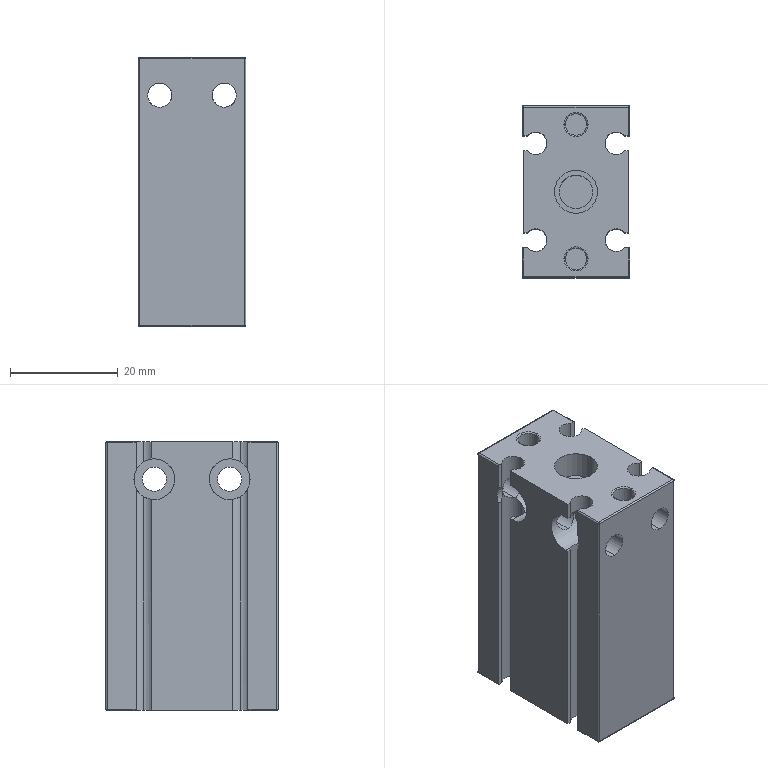Part | NX | features BREP 1 | 1 solid | 145 faces | box 20 x 32 x 50 mm | volume 22051 mm3 | cylinder 84 | plane 41 | torus 8 | sphere 8 | cone 4 | commonest cylinder face diameters 7.6 x20 0.5 x16 4.5 x16 4 x8 4.2 x8 1 x4